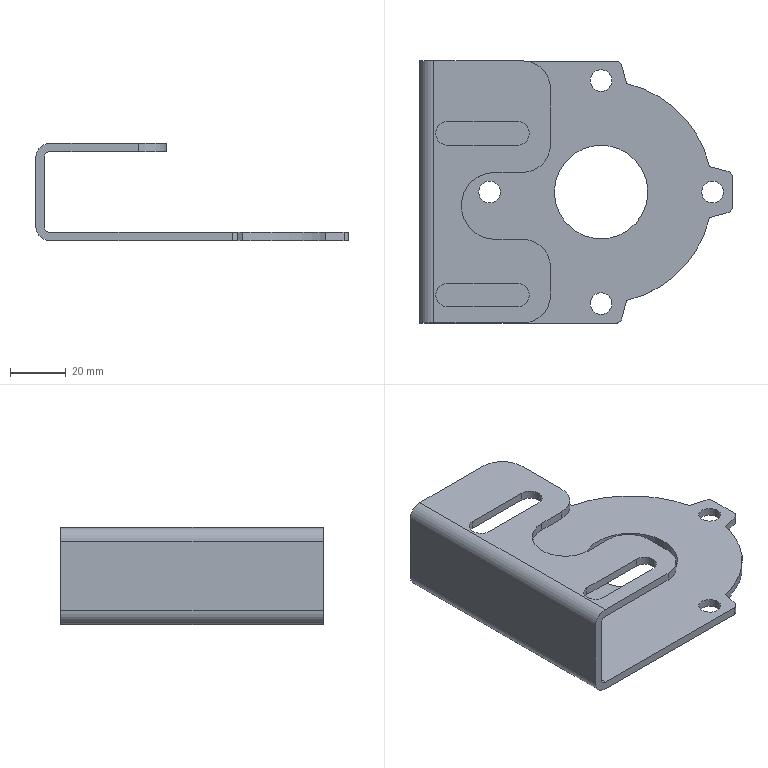Part | STEP file | S5 | 1 solid | 45 faces | box 112 x 94 x 34.858 mm | volume 39851 mm3 | cylinder 24 | plane 21 | commonest cylinder face diameters 4 x6 7.8 x4 8.5 x4 20 x4 10 x2 80 x2